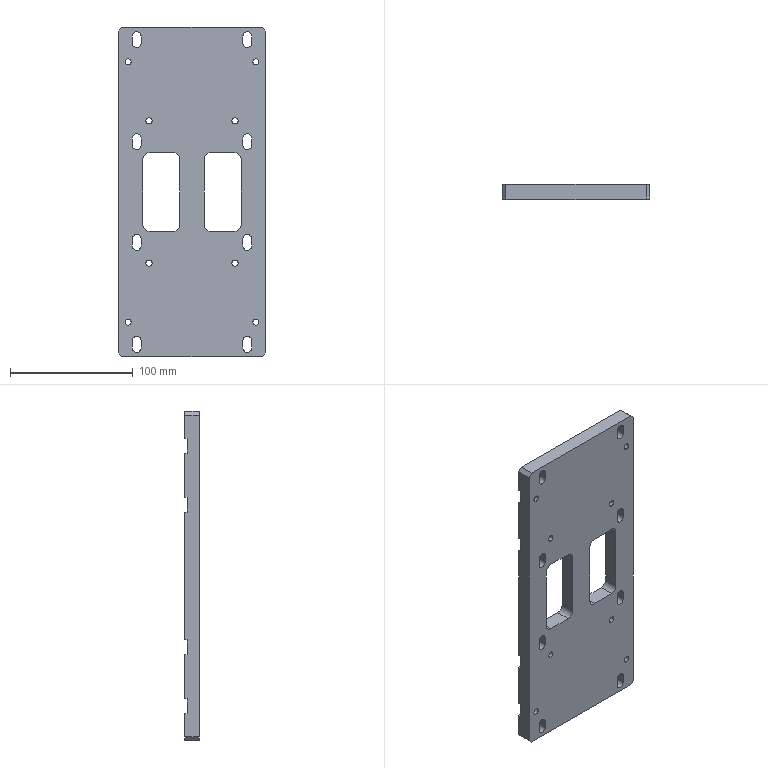Part | STEP file | (PA01.001.LX001) Wheel Train Base Plate | 1 solid | 98 faces | box 120 x 12 x 268 mm | volume 319322 mm3 | plane 50 | cylinder 48 | commonest cylinder face diameters 7 x24 5 x16 10 x8